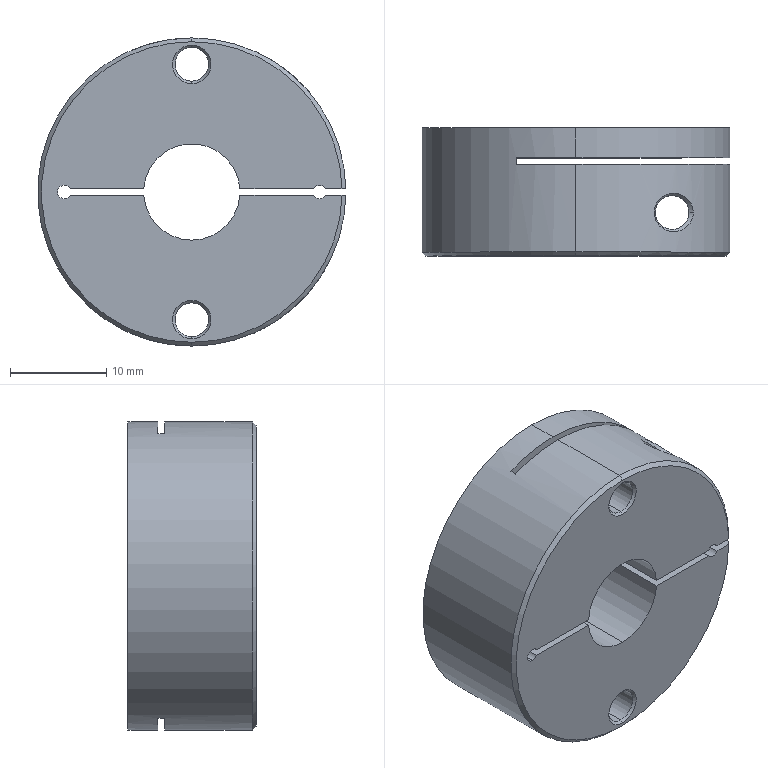Part | NX | 1 solid | 68 faces | box 31.996 x 13.3 x 32 mm | volume 8366 mm3 | cylinder 34 | plane 19 | cone 13 | spline 2 | commonest cylinder face diameters 3.5 x10 1.4 x9 10 x6 32 x5 4.5 x2 7.5 x2